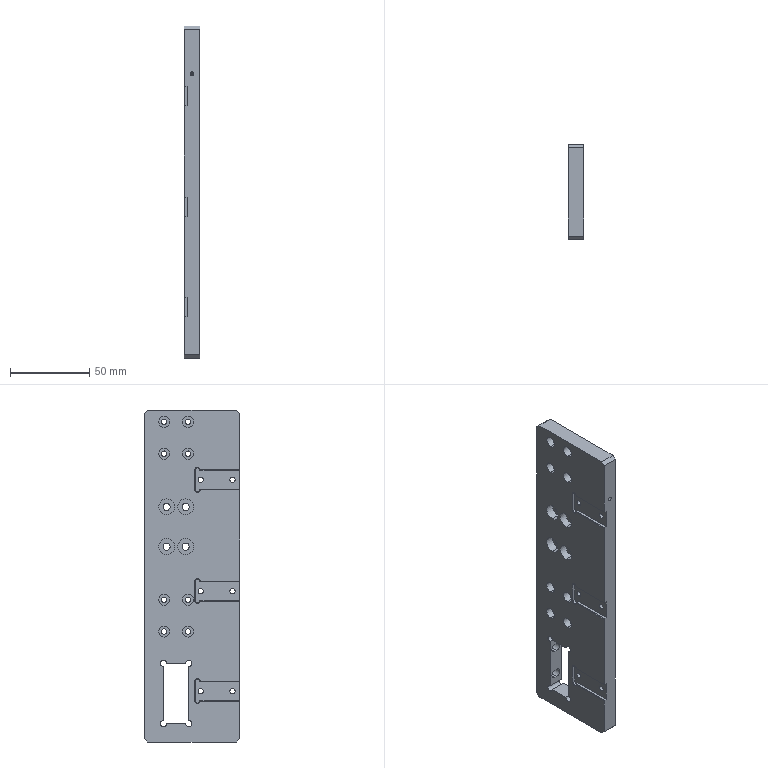Part | NX | features BREP 1 | 1 solid | 171 faces | box 10 x 60 x 209 mm | volume 110223 mm3 | cylinder 94 | plane 56 | cone 21 | commonest cylinder face diameters 3 x16 3.4 x16 7 x16 3.3 x12 2.5 x8 4.5 x8